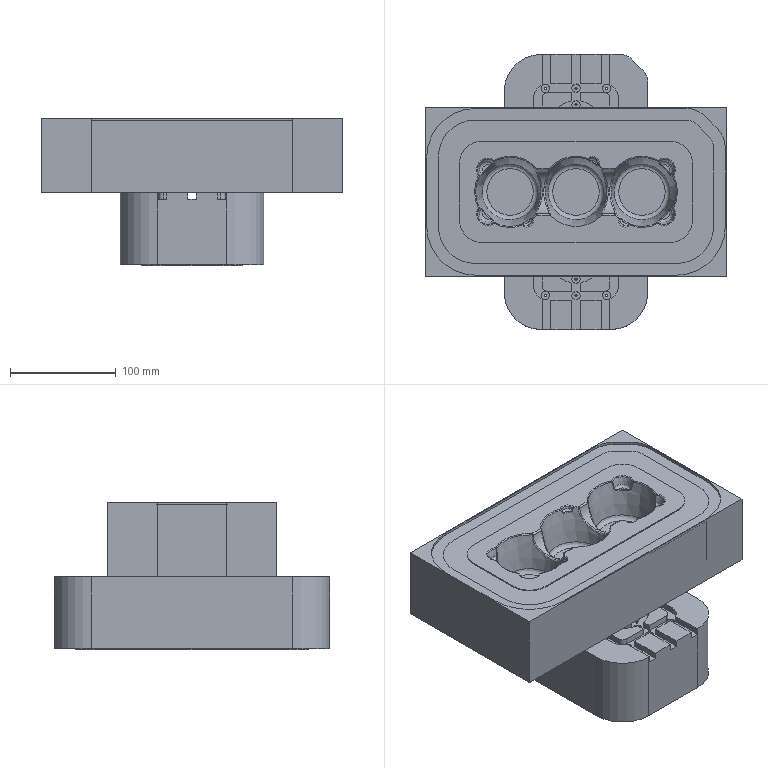Part | 4 solids | 615 faces | box 284.317 x 260.317 x 139.5 mm | volume 4696005 mm3 | plane 226 | cylinder 157 | spline 144 | torus 68 | cone 20 | commonest cylinder face diameters 2 x39 8 x39 31.81 x12 48.41 x12 70 x9 2.982 x8